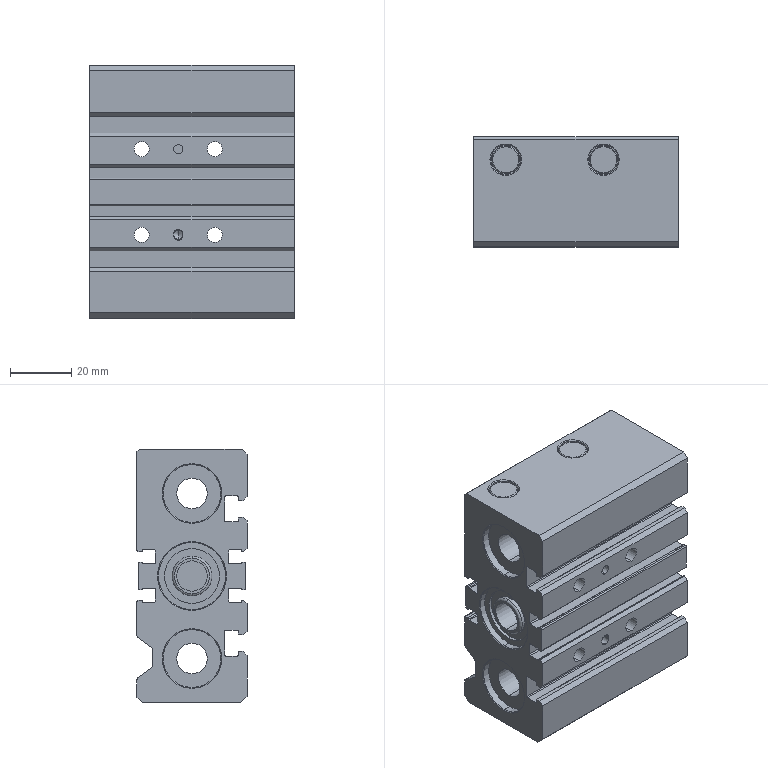Part | SolidWorks | features BaseBody 1 | 1 solid | 287 faces | box 67 x 36 x 83 mm | volume 131931 mm3 | cylinder 130 | plane 95 | cone 60 | torus 2 | commonest cylinder face diameters 0.8 x20 3 x14 0.4 x12 0.6 x10 4.134 x8 4.917 x8